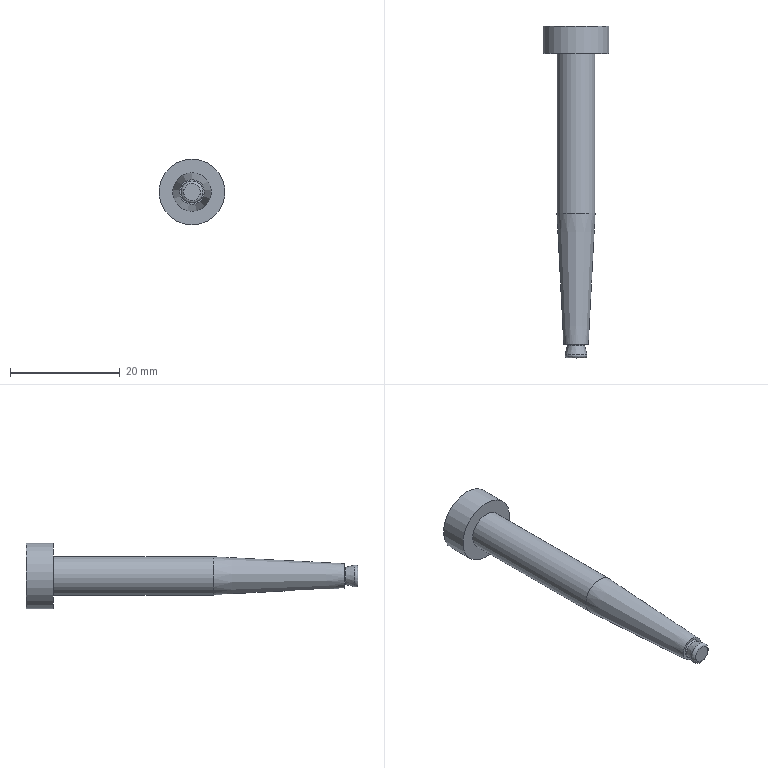Part | STEP file | RUNNER-PIN_id154_x_t | 1 solid | 10 faces | box 12 x 60.5 x 12 mm | volume 2342 mm3 | plane 4 | other 2 | cone 2 | cylinder 2 | commonest cylinder face diameters 7 x1 12 x1
STEP:
#1=CARTESIAN_POINT('',(-47.224,88.,17.945));
#2=VERTEX_POINT('',#1);
#3=CARTESIAN_POINT('',(-44.385,88.,16.866));
#4=VERTEX_POINT('',#3);
#5=CARTESIAN_POINT('',(-47.224,88.,17.945));
#6=CARTESIAN_POINT('',(-46.145,88.,20.783));
#7=CARTESIAN_POINT('',(-43.307,88.,19.705));
#8=CARTESIAN_POINT('',(-44.385,88.,16.866));
#9=(BOUNDED_CURVE()B_SPLINE_CURVE(3,(#5,#6,#7,#8),.UNSPECIFIED.,.F.,.F.)B_SPLINE_CURVE_WITH_KNOTS((4,4),(0.,1.),.UNSPECIFIED.)CURVE()GEOMETRIC_REPRESENTATION_ITEM()RATIONAL_B_SPLINE_CURVE((1.,0.3333,0.3333,1.))REPRESENTATION_ITEM(''));
#10=EDGE_CURVE('',#2,#4,#9,.T.);
#11=ORIENTED_EDGE('',*,*,#10,.F.);
#12=CARTESIAN_POINT('',(-44.385,88.,16.866));
#13=CARTESIAN_POINT('',(-45.464,88.,14.028));
#14=CARTESIAN_POINT('',(-48.302,88.,15.106));
#15=CARTESIAN_POINT('',(-47.224,88.,17.945));
#16=(BOUNDED_CURVE()B_SPLINE_CURVE(3,(#12,#13,#14,#15),.UNSPECIFIED.,.F.,.F.)B_SPLINE_CURVE_WITH_KNOTS((4,4),(0.,1.),.UNSPECIFIED.)CURVE()GEOMETRIC_REPRESENTATION_ITEM()RATIONAL_B_SPLINE_CURVE((1.,0.3333,0.3333,1.))REPRESENTATION_ITEM(''));
#17=EDGE_CURVE('',#4,#2,#16,.T.);
#18=ORIENTED_EDGE('',*,*,#17,.F.);
#19=EDGE_LOOP('',(#11,#18));
#20=FACE_OUTER_BOUND('',#19,.T.);
#21=CARTESIAN_POINT('',(-45.804,88.,17.406));
#22=DIRECTION('',(0.,1.,0.));
#23=DIRECTION('',(0.,0.,1.));
#24=AXIS2_PLACEMENT_3D('',#21,#22,#23);
#25=PLANE('',#24);
#26=ADVANCED_FACE('',(#20),#25,.F.);
#27=ORIENTED_EDGE('',*,*,#17,.T.);
#28=ORIENTED_EDGE('',*,*,#10,.T.);
#29=EDGE_LOOP('',(#27,#28));
#30=FACE_BOUND('',#29,.T.);
#31=CARTESIAN_POINT('',(-43.934,88.629,16.695));
#32=VERTEX_POINT('',#31);
#33=CARTESIAN_POINT('',(-45.804,88.629,17.406));
#34=DIRECTION('',(0.,1.,0.));
#35=DIRECTION('',(0.9348,0.,-0.3552));
#36=AXIS2_PLACEMENT_3D('',#33,#34,#35);
#37=CIRCLE('',#36,2.001);
#38=EDGE_CURVE('',#32,#32,#37,.T.);
#39=ORIENTED_EDGE('',*,*,#38,.F.);
#40=EDGE_LOOP('',(#39));
#41=FACE_BOUND('',#40,.T.);
#42=CARTESIAN_POINT('',(-47.224,88.5,17.945));
#43=DIRECTION('',(0.3552,0.,0.9348));
#44=DIRECTION('',(-0.9348,0.,0.3552));
#45=AXIS2_PLACEMENT_3D('',#42,#43,#44);
#46=CIRCLE('',#45,0.5);
#47=CARTESIAN_POINT('',(-45.804,88.5,17.406));
#48=DIRECTION('',(0.,1.,0.));
#49=AXIS1_PLACEMENT('',#47,#48);
#50=SURFACE_OF_REVOLUTION('',#46,#49);
#51=ADVANCED_FACE('',(#30,#41),#50,.F.);
#52=ORIENTED_EDGE('',*,*,#38,.T.);
#53=EDGE_LOOP('',(#52));
#54=FACE_BOUND('',#53,.T.);
#55=CARTESIAN_POINT('',(-47.27,90.248,17.962));
#56=VERTEX_POINT('',#55);
#57=CARTESIAN_POINT('',(-45.804,90.248,17.406));
#58=DIRECTION('',(0.,-1.,0.));
#59=DIRECTION('',(-0.9348,0.,0.3552));
#60=AXIS2_PLACEMENT_3D('',#57,#58,#59);
#61=CIRCLE('',#60,1.567);
#62=EDGE_CURVE('',#56,#56,#61,.T.);
#63=ORIENTED_EDGE('',*,*,#62,.T.);
#64=EDGE_LOOP('',(#63));
#65=FACE_BOUND('',#64,.T.);
#66=CARTESIAN_POINT('',(-45.804,88.629,17.406));
#67=DIRECTION('',(0.,-1.,0.));
#68=DIRECTION('',(0.,0.,-1.));
#69=AXIS2_PLACEMENT_3D('',#66,#67,#68);
#70=CONICAL_SURFACE('',#69,2.001,15.);
#71=ADVANCED_FACE('',(#54,#65),#70,.T.);
#72=ORIENTED_EDGE('',*,*,#62,.F.);
#73=EDGE_LOOP('',(#72));
#74=FACE_BOUND('',#73,.T.);
#75=CARTESIAN_POINT('',(-44.159,90.5,16.78));
#76=VERTEX_POINT('',#75);
#77=CARTESIAN_POINT('',(-47.45,90.5,18.031));
#78=VERTEX_POINT('',#77);
#79=CARTESIAN_POINT('',(-44.159,90.5,16.78));
#80=CARTESIAN_POINT('',(-42.908,90.5,20.072));
#81=CARTESIAN_POINT('',(-46.199,90.5,21.323));
#82=CARTESIAN_POINT('',(-47.45,90.5,18.031));
#83=(BOUNDED_CURVE()B_SPLINE_CURVE(3,(#79,#80,#81,#82),.UNSPECIFIED.,.F.,.F.)B_SPLINE_CURVE_WITH_KNOTS((4,4),(0.,1.),.UNSPECIFIED.)CURVE()GEOMETRIC_REPRESENTATION_ITEM()RATIONAL_B_SPLINE_CURVE((1.,0.3333,0.3333,1.))REPRESENTATION_ITEM(''));
#84=EDGE_CURVE('',#76,#78,#83,.T.);
#85=ORIENTED_EDGE('',*,*,#84,.T.);
#86=CARTESIAN_POINT('',(-47.45,90.5,18.031));
#87=CARTESIAN_POINT('',(-48.701,90.5,14.739));
#88=CARTESIAN_POINT('',(-45.409,90.5,13.489));
#89=CARTESIAN_POINT('',(-44.159,90.5,16.78));
#90=(BOUNDED_CURVE()B_SPLINE_CURVE(3,(#86,#87,#88,#89),.UNSPECIFIED.,.F.,.F.)B_SPLINE_CURVE_WITH_KNOTS((4,4),(0.,1.),.UNSPECIFIED.)CURVE()GEOMETRIC_REPRESENTATION_ITEM()RATIONAL_B_SPLINE_CURVE((1.,0.3333,0.3333,1.))REPRESENTATION_ITEM(''));
#91=EDGE_CURVE('',#78,#76,#90,.T.);
#92=ORIENTED_EDGE('',*,*,#91,.T.);
#93=EDGE_LOOP('',(#85,#92));
#94=FACE_BOUND('',#93,.T.);
#95=CARTESIAN_POINT('',(-47.45,90.3,18.031));
#96=DIRECTION('',(0.3552,0.,0.9348));
#97=DIRECTION('',(-0.9348,0.,0.3552));
#98=AXIS2_PLACEMENT_3D('',#95,#96,#97);
#99=CIRCLE('',#98,0.2);
#100=CARTESIAN_POINT('',(-45.804,90.3,17.406));
#101=DIRECTION('',(0.,1.,0.));
#102=AXIS1_PLACEMENT('',#100,#101);
#103=SURFACE_OF_REVOLUTION('',#99,#102);
#104=ADVANCED_FACE('',(#74,#94),#103,.T.);
#105=CARTESIAN_POINT('',(-45.804,148.5,23.406));
#106=VERTEX_POINT('',#105);
#107=CARTESIAN_POINT('',(-45.804,148.5,17.406));
#108=DIRECTION('',(0.,-1.,0.));
#109=DIRECTION('',(0.,0.,1.));
#110=AXIS2_PLACEMENT_3D('',#107,#108,#109);
#111=CIRCLE('',#110,6.);
#112=EDGE_CURVE('',#106,#106,#111,.T.);
#113=ORIENTED_EDGE('',*,*,#112,.F.);
#114=EDGE_LOOP('',(#113));
#115=FACE_OUTER_BOUND('',#114,.T.);
#116=CARTESIAN_POINT('',(-45.804,148.5,17.406));
#117=DIRECTION('',(0.,1.,0.));
#118=DIRECTION('',(0.,0.,1.));
#119=AXIS2_PLACEMENT_3D('',#116,#117,#118);
#120=PLANE('',#119);
#121=ADVANCED_FACE('',(#115),#120,.T.);
#122=ORIENTED_EDGE('',*,*,#91,.F.);
#123=ORIENTED_EDGE('',*,*,#84,.F.);
#124=EDGE_LOOP('',(#122,#123));
#125=FACE_BOUND('',#124,.T.);
#126=CARTESIAN_POINT('',(-45.804,90.5,19.656));
#127=VERTEX_POINT('',#126);
#128=CARTESIAN_POINT('',(-45.804,90.5,17.406));
#129=DIRECTION('',(0.,1.,0.));
#130=DIRECTION('',(0.,0.,1.));
#131=AXIS2_PLACEMENT_3D('',#128,#129,#130);
#132=CIRCLE('',#131,2.25);
#133=EDGE_CURVE('',#127,#127,#132,.T.);
#134=ORIENTED_EDGE('',*,*,#133,.F.);
#135=EDGE_LOOP('',(#134));
#136=FACE_BOUND('',#135,.T.);
#137=CARTESIAN_POINT('',(-45.804,90.5,17.406));
#138=DIRECTION('',(0.,1.,0.));
#139=DIRECTION('',(0.,0.,1.));
#140=AXIS2_PLACEMENT_3D('',#137,#138,#139);
#141=PLANE('',#140);
#142=ADVANCED_FACE('',(#125,#136),#141,.F.);
#143=ORIENTED_EDGE('',*,*,#112,.T.);
#144=EDGE_LOOP('',(#143));
#145=FACE_BOUND('',#144,.T.);
#146=CARTESIAN_POINT('',(-45.804,143.5,23.406));
#147=VERTEX_POINT('',#146);
#148=CARTESIAN_POINT('',(-45.804,143.5,17.406));
#149=DIRECTION('',(0.,1.,0.));
#150=DIRECTION('',(0.,0.,1.));
#151=AXIS2_PLACEMENT_3D('',#148,#149,#150);
#152=CIRCLE('',#151,6.);
#153=EDGE_CURVE('',#147,#147,#152,.T.);
#154=ORIENTED_EDGE('',*,*,#153,.T.);
#155=EDGE_LOOP('',(#154));
#156=FACE_BOUND('',#155,.T.);
#157=CARTESIAN_POINT('',(-45.804,84.975,17.406));
#158=DIRECTION('',(0.,1.,0.));
#159=DIRECTION('',(0.,0.,1.));
#160=AXIS2_PLACEMENT_3D('',#157,#158,#159);
#161=CYLINDRICAL_SURFACE('',#160,6.);
#162=ADVANCED_FACE('',(#145,#156),#161,.T.);
#163=CARTESIAN_POINT('',(-45.804,114.351,20.906));
#164=VERTEX_POINT('',#163);
#165=CARTESIAN_POINT('',(-45.804,114.351,17.406));
#166=DIRECTION('',(0.,1.,0.));
#167=DIRECTION('',(0.,0.,1.));
#168=AXIS2_PLACEMENT_3D('',#165,#166,#167);
#169=CIRCLE('',#168,3.5);
#170=EDGE_CURVE('',#164,#164,#169,.T.);
#171=ORIENTED_EDGE('',*,*,#170,.F.);
#172=EDGE_LOOP('',(#171));
#173=FACE_BOUND('',#172,.T.);
#174=ORIENTED_EDGE('',*,*,#133,.T.);
#175=EDGE_LOOP('',(#174));
#176=FACE_BOUND('',#175,.T.);
#177=CARTESIAN_POINT('',(-45.804,114.351,17.406));
#178=DIRECTION('',(0.,1.,0.));
#179=DIRECTION('',(0.,0.,1.));
#180=AXIS2_PLACEMENT_3D('',#177,#178,#179);
#181=CONICAL_SURFACE('',#180,3.5,3.);
#182=ADVANCED_FACE('',(#173,#176),#181,.T.);
#183=CARTESIAN_POINT('',(-45.804,143.5,20.906));
#184=VERTEX_POINT('',#183);
#185=CARTESIAN_POINT('',(-45.804,143.5,17.406));
#186=DIRECTION('',(0.,-1.,0.));
#187=DIRECTION('',(0.,0.,1.));
#188=AXIS2_PLACEMENT_3D('',#185,#186,#187);
#189=CIRCLE('',#188,3.5);
#190=EDGE_CURVE('',#184,#184,#189,.T.);
#191=ORIENTED_EDGE('',*,*,#190,.F.);
#192=EDGE_LOOP('',(#191));
#193=FACE_BOUND('',#192,.T.);
#194=ORIENTED_EDGE('',*,*,#153,.F.);
#195=EDGE_LOOP('',(#194));
#196=FACE_BOUND('',#195,.T.);
#197=CARTESIAN_POINT('',(-45.804,143.5,17.406));
#198=DIRECTION('',(0.,1.,0.));
#199=DIRECTION('',(0.,0.,1.));
#200=AXIS2_PLACEMENT_3D('',#197,#198,#199);
#201=PLANE('',#200);
#202=ADVANCED_FACE('',(#193,#196),#201,.F.);
#203=ORIENTED_EDGE('',*,*,#190,.T.);
#204=EDGE_LOOP('',(#203));
#205=FACE_BOUND('',#204,.T.);
#206=ORIENTED_EDGE('',*,*,#170,.T.);
#207=EDGE_LOOP('',(#206));
#208=FACE_BOUND('',#207,.T.);
#209=CARTESIAN_POINT('',(-45.804,84.975,17.406));
#210=DIRECTION('',(0.,1.,0.));
#211=DIRECTION('',(0.,0.,1.));
#212=AXIS2_PLACEMENT_3D('',#209,#210,#211);
#213=CYLINDRICAL_SURFACE('',#212,3.5);
#214=ADVANCED_FACE('',(#205,#208),#213,.T.);
#215=CLOSED_SHELL('',(#26,#51,#71,#104,#121,#142,#162,#182,#202,#214));
#216=MANIFOLD_SOLID_BREP('',#215);
#217=(LENGTH_UNIT()NAMED_UNIT(*)SI_UNIT(.MILLI.,.METRE.));
#218=UNCERTAINTY_MEASURE_WITH_UNIT(LENGTH_MEASURE(0.0508),#217,'','');
#219=(NAMED_UNIT(*)PLANE_ANGLE_UNIT()SI_UNIT($,.RADIAN.));
#220=PLANE_ANGLE_MEASURE_WITH_UNIT(PLANE_ANGLE_MEASURE(0.01745),#219);
#221=DIMENSIONAL_EXPONENTS(0.,0.,0.,0.,0.,0.,0.);
#222=(CONVERSION_BASED_UNIT('DEGREE',#220)NAMED_UNIT(#221)PLANE_ANGLE_UNIT());
#223=(NAMED_UNIT(*)SI_UNIT($,.STERADIAN.)SOLID_ANGLE_UNIT());
#224=(GEOMETRIC_REPRESENTATION_CONTEXT(3)GLOBAL_UNCERTAINTY_ASSIGNED_CONTEXT((#218))GLOBAL_UNIT_ASSIGNED_CONTEXT((#217,#222,#223))REPRESENTATION_CONTEXT('',''));
#225=ADVANCED_BREP_SHAPE_REPRESENTATION('',(#216),#224);